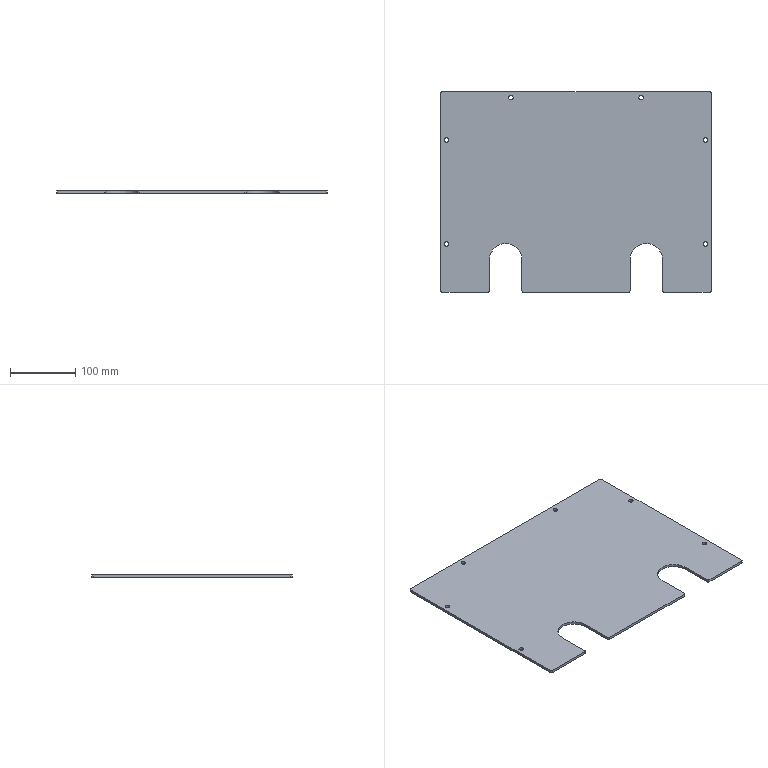Part | SolidWorks | features Fillet 2, HoleWzd 2, MirrorPattern 2, Extrusion 1, ICE 1 | 1 solid | 34 faces | box 416 x 308 x 4 mm | volume 483707 mm3 | cylinder 22 | plane 12 | commonest cylinder face diameters 7 x12 4 x8 50 x2
STEP:
#1=CARTESIAN_POINT('',(-103.5,145.,0.));
#2=VERTEX_POINT('',#1);
#3=CARTESIAN_POINT('',(-96.5,145.,0.));
#4=VERTEX_POINT('',#3);
#5=CARTESIAN_POINT('',(-100.,145.,0.));
#6=DIRECTION('',(0.,0.,1.));
#7=DIRECTION('',(1.,0.,0.));
#8=AXIS2_PLACEMENT_3D('',#5,#6,#7);
#9=CIRCLE('',#8,3.5);
#10=EDGE_CURVE('',#2,#4,#9,.T.);
#11=ORIENTED_EDGE('',*,*,#10,.F.);
#12=CARTESIAN_POINT('',(-103.5,145.,4.));
#13=VERTEX_POINT('',#12);
#14=CARTESIAN_POINT('',(-103.5,145.,4.));
#15=DIRECTION('',(0.,0.,1.));
#16=VECTOR('',#15,1000.);
#17=LINE('',#14,#16);
#18=EDGE_CURVE('',#2,#13,#17,.T.);
#19=ORIENTED_EDGE('',*,*,#18,.T.);
#20=CARTESIAN_POINT('',(-96.5,145.,4.));
#21=VERTEX_POINT('',#20);
#22=CARTESIAN_POINT('',(-100.,145.,4.));
#23=DIRECTION('',(0.,0.,1.));
#24=DIRECTION('',(1.,0.,0.));
#25=AXIS2_PLACEMENT_3D('',#22,#23,#24);
#26=CIRCLE('',#25,3.5);
#27=EDGE_CURVE('',#13,#21,#26,.T.);
#28=ORIENTED_EDGE('',*,*,#27,.T.);
#29=CARTESIAN_POINT('',(-96.5,145.,4.));
#30=DIRECTION('',(0.,0.,1.));
#31=VECTOR('',#30,1000.);
#32=LINE('',#29,#31);
#33=EDGE_CURVE('',#4,#21,#32,.T.);
#34=ORIENTED_EDGE('',*,*,#33,.F.);
#35=EDGE_LOOP('',(#11,#19,#28,#34));
#36=FACE_OUTER_BOUND('',#35,.T.);
#37=CARTESIAN_POINT('',(-100.,145.,4.));
#38=DIRECTION('',(0.,0.,1.));
#39=DIRECTION('',(1.,0.,0.));
#40=AXIS2_PLACEMENT_3D('',#37,#38,#39);
#41=CYLINDRICAL_SURFACE('',#40,3.5);
#42=ADVANCED_FACE('',(#36),#41,.F.);
#43=CARTESIAN_POINT('',(96.5,145.,0.));
#44=VERTEX_POINT('',#43);
#45=CARTESIAN_POINT('',(103.5,145.,0.));
#46=VERTEX_POINT('',#45);
#47=CARTESIAN_POINT('',(100.,145.,0.));
#48=DIRECTION('',(0.,0.,1.));
#49=DIRECTION('',(1.,0.,0.));
#50=AXIS2_PLACEMENT_3D('',#47,#48,#49);
#51=CIRCLE('',#50,3.5);
#52=EDGE_CURVE('',#44,#46,#51,.T.);
#53=ORIENTED_EDGE('',*,*,#52,.F.);
#54=CARTESIAN_POINT('',(96.5,145.,4.));
#55=VERTEX_POINT('',#54);
#56=CARTESIAN_POINT('',(96.5,145.,4.));
#57=DIRECTION('',(0.,0.,1.));
#58=VECTOR('',#57,1000.);
#59=LINE('',#56,#58);
#60=EDGE_CURVE('',#44,#55,#59,.T.);
#61=ORIENTED_EDGE('',*,*,#60,.T.);
#62=CARTESIAN_POINT('',(103.5,145.,4.));
#63=VERTEX_POINT('',#62);
#64=CARTESIAN_POINT('',(100.,145.,4.));
#65=DIRECTION('',(0.,0.,1.));
#66=DIRECTION('',(1.,0.,0.));
#67=AXIS2_PLACEMENT_3D('',#64,#65,#66);
#68=CIRCLE('',#67,3.5);
#69=EDGE_CURVE('',#55,#63,#68,.T.);
#70=ORIENTED_EDGE('',*,*,#69,.T.);
#71=CARTESIAN_POINT('',(103.5,145.,4.));
#72=DIRECTION('',(0.,0.,1.));
#73=VECTOR('',#72,1000.);
#74=LINE('',#71,#73);
#75=EDGE_CURVE('',#46,#63,#74,.T.);
#76=ORIENTED_EDGE('',*,*,#75,.F.);
#77=EDGE_LOOP('',(#53,#61,#70,#76));
#78=FACE_OUTER_BOUND('',#77,.T.);
#79=CARTESIAN_POINT('',(100.,145.,4.));
#80=DIRECTION('',(0.,0.,1.));
#81=DIRECTION('',(1.,0.,0.));
#82=AXIS2_PLACEMENT_3D('',#79,#80,#81);
#83=CYLINDRICAL_SURFACE('',#82,3.5);
#84=ADVANCED_FACE('',(#78),#83,.F.);
#85=CARTESIAN_POINT('',(195.5,80.,0.));
#86=VERTEX_POINT('',#85);
#87=CARTESIAN_POINT('',(202.5,80.,0.));
#88=VERTEX_POINT('',#87);
#89=CARTESIAN_POINT('',(199.,80.,0.));
#90=DIRECTION('',(0.,0.,1.));
#91=DIRECTION('',(1.,0.,0.));
#92=AXIS2_PLACEMENT_3D('',#89,#90,#91);
#93=CIRCLE('',#92,3.5);
#94=EDGE_CURVE('',#86,#88,#93,.T.);
#95=ORIENTED_EDGE('',*,*,#94,.F.);
#96=CARTESIAN_POINT('',(195.5,80.,4.));
#97=VERTEX_POINT('',#96);
#98=CARTESIAN_POINT('',(195.5,80.,4.));
#99=DIRECTION('',(0.,0.,1.));
#100=VECTOR('',#99,1000.);
#101=LINE('',#98,#100);
#102=EDGE_CURVE('',#86,#97,#101,.T.);
#103=ORIENTED_EDGE('',*,*,#102,.T.);
#104=CARTESIAN_POINT('',(202.5,80.,4.));
#105=VERTEX_POINT('',#104);
#106=CARTESIAN_POINT('',(199.,80.,4.));
#107=DIRECTION('',(0.,0.,1.));
#108=DIRECTION('',(1.,0.,0.));
#109=AXIS2_PLACEMENT_3D('',#106,#107,#108);
#110=CIRCLE('',#109,3.5);
#111=EDGE_CURVE('',#97,#105,#110,.T.);
#112=ORIENTED_EDGE('',*,*,#111,.T.);
#113=CARTESIAN_POINT('',(202.5,80.,4.));
#114=DIRECTION('',(0.,0.,1.));
#115=VECTOR('',#114,1000.);
#116=LINE('',#113,#115);
#117=EDGE_CURVE('',#88,#105,#116,.T.);
#118=ORIENTED_EDGE('',*,*,#117,.F.);
#119=EDGE_LOOP('',(#95,#103,#112,#118));
#120=FACE_OUTER_BOUND('',#119,.T.);
#121=CARTESIAN_POINT('',(199.,80.,4.));
#122=DIRECTION('',(0.,0.,1.));
#123=DIRECTION('',(1.,0.,0.));
#124=AXIS2_PLACEMENT_3D('',#121,#122,#123);
#125=CYLINDRICAL_SURFACE('',#124,3.5);
#126=ADVANCED_FACE('',(#120),#125,.F.);
#127=CARTESIAN_POINT('',(195.5,-80.,0.));
#128=VERTEX_POINT('',#127);
#129=CARTESIAN_POINT('',(202.5,-80.,0.));
#130=VERTEX_POINT('',#129);
#131=CARTESIAN_POINT('',(199.,-80.,0.));
#132=DIRECTION('',(0.,0.,1.));
#133=DIRECTION('',(1.,0.,0.));
#134=AXIS2_PLACEMENT_3D('',#131,#132,#133);
#135=CIRCLE('',#134,3.5);
#136=EDGE_CURVE('',#128,#130,#135,.T.);
#137=ORIENTED_EDGE('',*,*,#136,.F.);
#138=CARTESIAN_POINT('',(195.5,-80.,4.));
#139=VERTEX_POINT('',#138);
#140=CARTESIAN_POINT('',(195.5,-80.,4.));
#141=DIRECTION('',(0.,0.,1.));
#142=VECTOR('',#141,1000.);
#143=LINE('',#140,#142);
#144=EDGE_CURVE('',#128,#139,#143,.T.);
#145=ORIENTED_EDGE('',*,*,#144,.T.);
#146=CARTESIAN_POINT('',(202.5,-80.,4.));
#147=VERTEX_POINT('',#146);
#148=CARTESIAN_POINT('',(199.,-80.,4.));
#149=DIRECTION('',(0.,0.,1.));
#150=DIRECTION('',(1.,0.,0.));
#151=AXIS2_PLACEMENT_3D('',#148,#149,#150);
#152=CIRCLE('',#151,3.5);
#153=EDGE_CURVE('',#139,#147,#152,.T.);
#154=ORIENTED_EDGE('',*,*,#153,.T.);
#155=CARTESIAN_POINT('',(202.5,-80.,4.));
#156=DIRECTION('',(0.,0.,1.));
#157=VECTOR('',#156,1000.);
#158=LINE('',#155,#157);
#159=EDGE_CURVE('',#130,#147,#158,.T.);
#160=ORIENTED_EDGE('',*,*,#159,.F.);
#161=EDGE_LOOP('',(#137,#145,#154,#160));
#162=FACE_OUTER_BOUND('',#161,.T.);
#163=CARTESIAN_POINT('',(199.,-80.,4.));
#164=DIRECTION('',(0.,0.,1.));
#165=DIRECTION('',(1.,0.,0.));
#166=AXIS2_PLACEMENT_3D('',#163,#164,#165);
#167=CYLINDRICAL_SURFACE('',#166,3.5);
#168=ADVANCED_FACE('',(#162),#167,.F.);
#169=CARTESIAN_POINT('',(-202.5,80.,0.));
#170=VERTEX_POINT('',#169);
#171=CARTESIAN_POINT('',(-195.5,80.,0.));
#172=VERTEX_POINT('',#171);
#173=CARTESIAN_POINT('',(-199.,80.,0.));
#174=DIRECTION('',(0.,0.,1.));
#175=DIRECTION('',(1.,0.,0.));
#176=AXIS2_PLACEMENT_3D('',#173,#174,#175);
#177=CIRCLE('',#176,3.5);
#178=EDGE_CURVE('',#170,#172,#177,.T.);
#179=ORIENTED_EDGE('',*,*,#178,.F.);
#180=CARTESIAN_POINT('',(-202.5,80.,4.));
#181=VERTEX_POINT('',#180);
#182=CARTESIAN_POINT('',(-202.5,80.,4.));
#183=DIRECTION('',(0.,0.,1.));
#184=VECTOR('',#183,1000.);
#185=LINE('',#182,#184);
#186=EDGE_CURVE('',#170,#181,#185,.T.);
#187=ORIENTED_EDGE('',*,*,#186,.T.);
#188=CARTESIAN_POINT('',(-195.5,80.,4.));
#189=VERTEX_POINT('',#188);
#190=CARTESIAN_POINT('',(-199.,80.,4.));
#191=DIRECTION('',(0.,0.,1.));
#192=DIRECTION('',(1.,0.,0.));
#193=AXIS2_PLACEMENT_3D('',#190,#191,#192);
#194=CIRCLE('',#193,3.5);
#195=EDGE_CURVE('',#181,#189,#194,.T.);
#196=ORIENTED_EDGE('',*,*,#195,.T.);
#197=CARTESIAN_POINT('',(-195.5,80.,4.));
#198=DIRECTION('',(0.,0.,1.));
#199=VECTOR('',#198,1000.);
#200=LINE('',#197,#199);
#201=EDGE_CURVE('',#172,#189,#200,.T.);
#202=ORIENTED_EDGE('',*,*,#201,.F.);
#203=EDGE_LOOP('',(#179,#187,#196,#202));
#204=FACE_OUTER_BOUND('',#203,.T.);
#205=CARTESIAN_POINT('',(-199.,80.,4.));
#206=DIRECTION('',(0.,0.,1.));
#207=DIRECTION('',(1.,0.,0.));
#208=AXIS2_PLACEMENT_3D('',#205,#206,#207);
#209=CYLINDRICAL_SURFACE('',#208,3.5);
#210=ADVANCED_FACE('',(#204),#209,.F.);
#211=CARTESIAN_POINT('',(-202.5,-80.,0.));
#212=VERTEX_POINT('',#211);
#213=CARTESIAN_POINT('',(-195.5,-80.,0.));
#214=VERTEX_POINT('',#213);
#215=CARTESIAN_POINT('',(-199.,-80.,0.));
#216=DIRECTION('',(0.,0.,1.));
#217=DIRECTION('',(1.,0.,0.));
#218=AXIS2_PLACEMENT_3D('',#215,#216,#217);
#219=CIRCLE('',#218,3.5);
#220=EDGE_CURVE('',#212,#214,#219,.T.);
#221=ORIENTED_EDGE('',*,*,#220,.F.);
#222=CARTESIAN_POINT('',(-202.5,-80.,4.));
#223=VERTEX_POINT('',#222);
#224=CARTESIAN_POINT('',(-202.5,-80.,4.));
#225=DIRECTION('',(0.,0.,1.));
#226=VECTOR('',#225,1000.);
#227=LINE('',#224,#226);
#228=EDGE_CURVE('',#212,#223,#227,.T.);
#229=ORIENTED_EDGE('',*,*,#228,.T.);
#230=CARTESIAN_POINT('',(-195.5,-80.,4.));
#231=VERTEX_POINT('',#230);
#232=CARTESIAN_POINT('',(-199.,-80.,4.));
#233=DIRECTION('',(0.,0.,1.));
#234=DIRECTION('',(1.,0.,0.));
#235=AXIS2_PLACEMENT_3D('',#232,#233,#234);
#236=CIRCLE('',#235,3.5);
#237=EDGE_CURVE('',#223,#231,#236,.T.);
#238=ORIENTED_EDGE('',*,*,#237,.T.);
#239=CARTESIAN_POINT('',(-195.5,-80.,4.));
#240=DIRECTION('',(0.,0.,1.));
#241=VECTOR('',#240,1000.);
#242=LINE('',#239,#241);
#243=EDGE_CURVE('',#214,#231,#242,.T.);
#244=ORIENTED_EDGE('',*,*,#243,.F.);
#245=EDGE_LOOP('',(#221,#229,#238,#244));
#246=FACE_OUTER_BOUND('',#245,.T.);
#247=CARTESIAN_POINT('',(-199.,-80.,4.));
#248=DIRECTION('',(0.,0.,1.));
#249=DIRECTION('',(1.,0.,0.));
#250=AXIS2_PLACEMENT_3D('',#247,#248,#249);
#251=CYLINDRICAL_SURFACE('',#250,3.5);
#252=ADVANCED_FACE('',(#246),#251,.F.);
#253=CARTESIAN_POINT('',(-81.,-154.,0.));
#254=VERTEX_POINT('',#253);
#255=CARTESIAN_POINT('',(81.,-154.,0.));
#256=VERTEX_POINT('',#255);
#257=CARTESIAN_POINT('',(208.,-154.,0.));
#258=DIRECTION('',(1.,0.,0.));
#259=VECTOR('',#258,1000.);
#260=LINE('',#257,#259);
#261=EDGE_CURVE('',#254,#256,#260,.T.);
#262=ORIENTED_EDGE('',*,*,#261,.T.);
#263=CARTESIAN_POINT('',(81.,-154.,4.));
#264=VERTEX_POINT('',#263);
#265=CARTESIAN_POINT('',(81.,-154.,4.));
#266=DIRECTION('',(0.,0.,1.));
#267=VECTOR('',#266,1000.);
#268=LINE('',#265,#267);
#269=EDGE_CURVE('',#256,#264,#268,.T.);
#270=ORIENTED_EDGE('',*,*,#269,.T.);
#271=CARTESIAN_POINT('',(-81.,-154.,4.));
#272=VERTEX_POINT('',#271);
#273=CARTESIAN_POINT('',(208.,-154.,4.));
#274=DIRECTION('',(1.,0.,0.));
#275=VECTOR('',#274,1000.);
#276=LINE('',#273,#275);
#277=EDGE_CURVE('',#272,#264,#276,.T.);
#278=ORIENTED_EDGE('',*,*,#277,.F.);
#279=CARTESIAN_POINT('',(-81.,-154.,4.));
#280=DIRECTION('',(0.,0.,-1.));
#281=VECTOR('',#280,1000.);
#282=LINE('',#279,#281);
#283=EDGE_CURVE('',#272,#254,#282,.T.);
#284=ORIENTED_EDGE('',*,*,#283,.T.);
#285=EDGE_LOOP('',(#262,#270,#278,#284));
#286=FACE_OUTER_BOUND('',#285,.T.);
#287=CARTESIAN_POINT('',(208.,-154.,4.));
#288=DIRECTION('',(0.,1.,0.));
#289=DIRECTION('',(-1.,0.,0.));
#290=AXIS2_PLACEMENT_3D('',#287,#288,#289);
#291=PLANE('',#290);
#292=ADVANCED_FACE('',(#286),#291,.F.);
#293=CARTESIAN_POINT('',(135.,-154.,4.));
#294=VERTEX_POINT('',#293);
#295=CARTESIAN_POINT('',(206.,-154.,4.));
#296=VERTEX_POINT('',#295);
#297=CARTESIAN_POINT('',(208.,-154.,4.));
#298=DIRECTION('',(1.,0.,0.));
#299=VECTOR('',#298,1000.);
#300=LINE('',#297,#299);
#301=EDGE_CURVE('',#294,#296,#300,.T.);
#302=ORIENTED_EDGE('',*,*,#301,.F.);
#303=CARTESIAN_POINT('',(135.,-154.,0.));
#304=VERTEX_POINT('',#303);
#305=CARTESIAN_POINT('',(135.,-154.,0.));
#306=DIRECTION('',(0.,0.,-1.));
#307=VECTOR('',#306,1000.);
#308=LINE('',#305,#307);
#309=EDGE_CURVE('',#294,#304,#308,.T.);
#310=ORIENTED_EDGE('',*,*,#309,.T.);
#311=CARTESIAN_POINT('',(206.,-154.,0.));
#312=VERTEX_POINT('',#311);
#313=CARTESIAN_POINT('',(208.,-154.,0.));
#314=DIRECTION('',(1.,0.,0.));
#315=VECTOR('',#314,1000.);
#316=LINE('',#313,#315);
#317=EDGE_CURVE('',#304,#312,#316,.T.);
#318=ORIENTED_EDGE('',*,*,#317,.T.);
#319=CARTESIAN_POINT('',(206.,-154.,4.));
#320=DIRECTION('',(0.,0.,1.));
#321=VECTOR('',#320,1000.);
#322=LINE('',#319,#321);
#323=EDGE_CURVE('',#312,#296,#322,.T.);
#324=ORIENTED_EDGE('',*,*,#323,.T.);
#325=EDGE_LOOP('',(#302,#310,#318,#324));
#326=FACE_OUTER_BOUND('',#325,.T.);
#327=CARTESIAN_POINT('',(208.,-154.,4.));
#328=DIRECTION('',(0.,1.,0.));
#329=DIRECTION('',(-1.,0.,0.));
#330=AXIS2_PLACEMENT_3D('',#327,#328,#329);
#331=PLANE('',#330);
#332=ADVANCED_FACE('',(#326),#331,.F.);
#333=CARTESIAN_POINT('',(-100.,145.,4.));
#334=DIRECTION('',(0.,0.,1.));
#335=DIRECTION('',(1.,0.,0.));
#336=AXIS2_PLACEMENT_3D('',#333,#334,#335);
#337=CIRCLE('',#336,3.5);
#338=EDGE_CURVE('',#21,#13,#337,.T.);
#339=ORIENTED_EDGE('',*,*,#338,.F.);
#340=ORIENTED_EDGE('',*,*,#27,.F.);
#341=EDGE_LOOP('',(#339,#340));
#342=FACE_BOUND('',#341,.T.);
#343=CARTESIAN_POINT('',(100.,145.,4.));
#344=DIRECTION('',(0.,0.,1.));
#345=DIRECTION('',(1.,0.,0.));
#346=AXIS2_PLACEMENT_3D('',#343,#344,#345);
#347=CIRCLE('',#346,3.5);
#348=EDGE_CURVE('',#63,#55,#347,.T.);
#349=ORIENTED_EDGE('',*,*,#348,.F.);
#350=ORIENTED_EDGE('',*,*,#69,.F.);
#351=EDGE_LOOP('',(#349,#350));
#352=FACE_BOUND('',#351,.T.);
#353=CARTESIAN_POINT('',(199.,80.,4.));
#354=DIRECTION('',(0.,0.,1.));
#355=DIRECTION('',(1.,0.,0.));
#356=AXIS2_PLACEMENT_3D('',#353,#354,#355);
#357=CIRCLE('',#356,3.5);
#358=EDGE_CURVE('',#105,#97,#357,.T.);
#359=ORIENTED_EDGE('',*,*,#358,.F.);
#360=ORIENTED_EDGE('',*,*,#111,.F.);
#361=EDGE_LOOP('',(#359,#360));
#362=FACE_BOUND('',#361,.T.);
#363=CARTESIAN_POINT('',(199.,-80.,4.));
#364=DIRECTION('',(0.,0.,1.));
#365=DIRECTION('',(1.,0.,0.));
#366=AXIS2_PLACEMENT_3D('',#363,#364,#365);
#367=CIRCLE('',#366,3.5);
#368=EDGE_CURVE('',#147,#139,#367,.T.);
#369=ORIENTED_EDGE('',*,*,#368,.F.);
#370=ORIENTED_EDGE('',*,*,#153,.F.);
#371=EDGE_LOOP('',(#369,#370));
#372=FACE_BOUND('',#371,.T.);
#373=CARTESIAN_POINT('',(-199.,80.,4.));
#374=DIRECTION('',(0.,0.,1.));
#375=DIRECTION('',(1.,0.,0.));
#376=AXIS2_PLACEMENT_3D('',#373,#374,#375);
#377=CIRCLE('',#376,3.5);
#378=EDGE_CURVE('',#189,#181,#377,.T.);
#379=ORIENTED_EDGE('',*,*,#378,.F.);
#380=ORIENTED_EDGE('',*,*,#195,.F.);
#381=EDGE_LOOP('',(#379,#380));
#382=FACE_BOUND('',#381,.T.);
#383=CARTESIAN_POINT('',(-199.,-80.,4.));
#384=DIRECTION('',(0.,0.,1.));
#385=DIRECTION('',(1.,0.,0.));
#386=AXIS2_PLACEMENT_3D('',#383,#384,#385);
#387=CIRCLE('',#386,3.5);
#388=EDGE_CURVE('',#231,#223,#387,.T.);
#389=ORIENTED_EDGE('',*,*,#388,.F.);
#390=ORIENTED_EDGE('',*,*,#237,.F.);
#391=EDGE_LOOP('',(#389,#390));
#392=FACE_BOUND('',#391,.T.);
#393=CARTESIAN_POINT('',(133.,-104.,4.));
#394=VERTEX_POINT('',#393);
#395=CARTESIAN_POINT('',(133.,-152.,4.));
#396=VERTEX_POINT('',#395);
#397=CARTESIAN_POINT('',(133.,-154.,4.));
#398=DIRECTION('',(0.,-1.,0.));
#399=VECTOR('',#398,1000.);
#400=LINE('',#397,#399);
#401=EDGE_CURVE('',#394,#396,#400,.T.);
#402=ORIENTED_EDGE('',*,*,#401,.T.);
#403=CARTESIAN_POINT('',(135.,-152.,4.));
#404=DIRECTION('',(0.,0.,1.));
#405=DIRECTION('',(1.,0.,0.));
#406=AXIS2_PLACEMENT_3D('',#403,#404,#405);
#407=CIRCLE('',#406,2.);
#408=EDGE_CURVE('',#396,#294,#407,.T.);
#409=ORIENTED_EDGE('',*,*,#408,.T.);
#410=ORIENTED_EDGE('',*,*,#301,.T.);
#411=CARTESIAN_POINT('',(208.,-152.,4.));
#412=VERTEX_POINT('',#411);
#413=CARTESIAN_POINT('',(206.,-152.,4.));
#414=DIRECTION('',(0.,0.,1.));
#415=DIRECTION('',(1.,0.,0.));
#416=AXIS2_PLACEMENT_3D('',#413,#414,#415);
#417=CIRCLE('',#416,2.);
#418=EDGE_CURVE('',#296,#412,#417,.T.);
#419=ORIENTED_EDGE('',*,*,#418,.T.);
#420=CARTESIAN_POINT('',(208.,152.,4.));
#421=VERTEX_POINT('',#420);
#422=CARTESIAN_POINT('',(208.,-154.,4.));
#423=DIRECTION('',(0.,1.,0.));
#424=VECTOR('',#423,1000.);
#425=LINE('',#422,#424);
#426=EDGE_CURVE('',#412,#421,#425,.T.);
#427=ORIENTED_EDGE('',*,*,#426,.T.);
#428=CARTESIAN_POINT('',(206.,154.,4.));
#429=VERTEX_POINT('',#428);
#430=CARTESIAN_POINT('',(206.,152.,4.));
#431=DIRECTION('',(0.,0.,1.));
#432=DIRECTION('',(1.,0.,0.));
#433=AXIS2_PLACEMENT_3D('',#430,#431,#432);
#434=CIRCLE('',#433,2.);
#435=EDGE_CURVE('',#421,#429,#434,.T.);
#436=ORIENTED_EDGE('',*,*,#435,.T.);
#437=CARTESIAN_POINT('',(-206.,154.,4.));
#438=VERTEX_POINT('',#437);
#439=CARTESIAN_POINT('',(208.,154.,4.));
#440=DIRECTION('',(-1.,0.,0.));
#441=VECTOR('',#440,1000.);
#442=LINE('',#439,#441);
#443=EDGE_CURVE('',#429,#438,#442,.T.);
#444=ORIENTED_EDGE('',*,*,#443,.T.);
#445=CARTESIAN_POINT('',(-208.,152.,4.));
#446=VERTEX_POINT('',#445);
#447=CARTESIAN_POINT('',(-206.,152.,4.));
#448=DIRECTION('',(0.,0.,1.));
#449=DIRECTION('',(1.,0.,0.));
#450=AXIS2_PLACEMENT_3D('',#447,#448,#449);
#451=CIRCLE('',#450,2.);
#452=EDGE_CURVE('',#438,#446,#451,.T.);
#453=ORIENTED_EDGE('',*,*,#452,.T.);
#454=CARTESIAN_POINT('',(-208.,-152.,4.));
#455=VERTEX_POINT('',#454);
#456=CARTESIAN_POINT('',(-208.,-154.,4.));
#457=DIRECTION('',(0.,-1.,0.));
#458=VECTOR('',#457,1000.);
#459=LINE('',#456,#458);
#460=EDGE_CURVE('',#446,#455,#459,.T.);
#461=ORIENTED_EDGE('',*,*,#460,.T.);
#462=CARTESIAN_POINT('',(-206.,-154.,4.));
#463=VERTEX_POINT('',#462);
#464=CARTESIAN_POINT('',(-206.,-152.,4.));
#465=DIRECTION('',(0.,0.,1.));
#466=DIRECTION('',(1.,0.,0.));
#467=AXIS2_PLACEMENT_3D('',#464,#465,#466);
#468=CIRCLE('',#467,2.);
#469=EDGE_CURVE('',#455,#463,#468,.T.);
#470=ORIENTED_EDGE('',*,*,#469,.T.);
#471=CARTESIAN_POINT('',(-135.,-154.,4.));
#472=VERTEX_POINT('',#471);
#473=CARTESIAN_POINT('',(208.,-154.,4.));
#474=DIRECTION('',(1.,0.,0.));
#475=VECTOR('',#474,1000.);
#476=LINE('',#473,#475);
#477=EDGE_CURVE('',#463,#472,#476,.T.);
#478=ORIENTED_EDGE('',*,*,#477,.T.);
#479=CARTESIAN_POINT('',(-133.,-152.,4.));
#480=VERTEX_POINT('',#479);
#481=CARTESIAN_POINT('',(-135.,-152.,4.));
#482=DIRECTION('',(0.,0.,1.));
#483=DIRECTION('',(1.,0.,0.));
#484=AXIS2_PLACEMENT_3D('',#481,#482,#483);
#485=CIRCLE('',#484,2.);
#486=EDGE_CURVE('',#472,#480,#485,.T.);
#487=ORIENTED_EDGE('',*,*,#486,.T.);
#488=CARTESIAN_POINT('',(-133.,-104.,4.));
#489=VERTEX_POINT('',#488);
#490=CARTESIAN_POINT('',(-133.,-154.,4.));
#491=DIRECTION('',(0.,-1.,0.));
#492=VECTOR('',#491,1000.);
#493=LINE('',#490,#492);
#494=EDGE_CURVE('',#489,#480,#493,.T.);
#495=ORIENTED_EDGE('',*,*,#494,.F.);
#496=CARTESIAN_POINT('',(-83.,-104.,4.));
#497=VERTEX_POINT('',#496);
#498=CARTESIAN_POINT('',(-108.,-104.,4.));
#499=DIRECTION('',(0.,0.,1.));
#500=DIRECTION('',(1.,0.,0.));
#501=AXIS2_PLACEMENT_3D('',#498,#499,#500);
#502=CIRCLE('',#501,25.);
#503=EDGE_CURVE('',#497,#489,#502,.T.);
#504=ORIENTED_EDGE('',*,*,#503,.F.);
#505=CARTESIAN_POINT('',(-83.,-152.,4.));
#506=VERTEX_POINT('',#505);
#507=CARTESIAN_POINT('',(-83.,-154.,4.));
#508=DIRECTION('',(0.,1.,0.));
#509=VECTOR('',#508,1000.);
#510=LINE('',#507,#509);
#511=EDGE_CURVE('',#506,#497,#510,.T.);
#512=ORIENTED_EDGE('',*,*,#511,.F.);
#513=CARTESIAN_POINT('',(-81.,-152.,4.));
#514=DIRECTION('',(0.,0.,1.));
#515=DIRECTION('',(1.,0.,0.));
#516=AXIS2_PLACEMENT_3D('',#513,#514,#515);
#517=CIRCLE('',#516,2.);
#518=EDGE_CURVE('',#506,#272,#517,.T.);
#519=ORIENTED_EDGE('',*,*,#518,.T.);
#520=ORIENTED_EDGE('',*,*,#277,.T.);
#521=CARTESIAN_POINT('',(83.,-152.,4.));
#522=VERTEX_POINT('',#521);
#523=CARTESIAN_POINT('',(81.,-152.,4.));
#524=DIRECTION('',(0.,0.,1.));
#525=DIRECTION('',(1.,0.,0.));
#526=AXIS2_PLACEMENT_3D('',#523,#524,#525);
#527=CIRCLE('',#526,2.);
#528=EDGE_CURVE('',#264,#522,#527,.T.);
#529=ORIENTED_EDGE('',*,*,#528,.T.);
#530=CARTESIAN_POINT('',(83.,-104.,4.));
#531=VERTEX_POINT('',#530);
#532=CARTESIAN_POINT('',(83.,-154.,4.));
#533=DIRECTION('',(0.,1.,0.));
#534=VECTOR('',#533,1000.);
#535=LINE('',#532,#534);
#536=EDGE_CURVE('',#522,#531,#535,.T.);
#537=ORIENTED_EDGE('',*,*,#536,.T.);
#538=CARTESIAN_POINT('',(108.,-104.,4.));
#539=DIRECTION('',(0.,0.,-1.));
#540=DIRECTION('',(-1.,0.,0.));
#541=AXIS2_PLACEMENT_3D('',#538,#539,#540);
#542=CIRCLE('',#541,25.);
#543=EDGE_CURVE('',#531,#394,#542,.T.);
#544=ORIENTED_EDGE('',*,*,#543,.T.);
#545=EDGE_LOOP('',(#402,#409,#410,#419,#427,#436,#444,#453,#461,#470,#478,#487,#495,#504,#512,#519,#520,#529,#537,#544));
#546=FACE_OUTER_BOUND('',#545,.T.);
#547=CARTESIAN_POINT('',(0.,0.,4.));
#548=DIRECTION('',(0.,0.,1.));
#549=DIRECTION('',(1.,0.,0.));
#550=AXIS2_PLACEMENT_3D('',#547,#548,#549);
#551=PLANE('',#550);
#552=ADVANCED_FACE('',(#342,#352,#362,#372,#382,#392,#546),#551,.T.);
#553=CARTESIAN_POINT('',(-100.,145.,0.));
#554=DIRECTION('',(0.,0.,1.));
#555=DIRECTION('',(1.,0.,0.));
#556=AXIS2_PLACEMENT_3D('',#553,#554,#555);
#557=CIRCLE('',#556,3.5);
#558=EDGE_CURVE('',#4,#2,#557,.T.);
#559=ORIENTED_EDGE('',*,*,#558,.T.);
#560=ORIENTED_EDGE('',*,*,#10,.T.);
#561=EDGE_LOOP('',(#559,#560));
#562=FACE_BOUND('',#561,.T.);
#563=CARTESIAN_POINT('',(100.,145.,0.));
#564=DIRECTION('',(0.,0.,1.));
#565=DIRECTION('',(1.,0.,0.));
#566=AXIS2_PLACEMENT_3D('',#563,#564,#565);
#567=CIRCLE('',#566,3.5);
#568=EDGE_CURVE('',#46,#44,#567,.T.);
#569=ORIENTED_EDGE('',*,*,#568,.T.);
#570=ORIENTED_EDGE('',*,*,#52,.T.);
#571=EDGE_LOOP('',(#569,#570));
#572=FACE_BOUND('',#571,.T.);
#573=CARTESIAN_POINT('',(199.,80.,0.));
#574=DIRECTION('',(0.,0.,1.));
#575=DIRECTION('',(1.,0.,0.));
#576=AXIS2_PLACEMENT_3D('',#573,#574,#575);
#577=CIRCLE('',#576,3.5);
#578=EDGE_CURVE('',#88,#86,#577,.T.);
#579=ORIENTED_EDGE('',*,*,#578,.T.);
#580=ORIENTED_EDGE('',*,*,#94,.T.);
#581=EDGE_LOOP('',(#579,#580));
#582=FACE_BOUND('',#581,.T.);
#583=CARTESIAN_POINT('',(199.,-80.,0.));
#584=DIRECTION('',(0.,0.,1.));
#585=DIRECTION('',(1.,0.,0.));
#586=AXIS2_PLACEMENT_3D('',#583,#584,#585);
#587=CIRCLE('',#586,3.5);
#588=EDGE_CURVE('',#130,#128,#587,.T.);
#589=ORIENTED_EDGE('',*,*,#588,.T.);
#590=ORIENTED_EDGE('',*,*,#136,.T.);
#591=EDGE_LOOP('',(#589,#590));
#592=FACE_BOUND('',#591,.T.);
#593=CARTESIAN_POINT('',(-199.,80.,0.));
#594=DIRECTION('',(0.,0.,1.));
#595=DIRECTION('',(1.,0.,0.));
#596=AXIS2_PLACEMENT_3D('',#593,#594,#595);
#597=CIRCLE('',#596,3.5);
#598=EDGE_CURVE('',#172,#170,#597,.T.);
#599=ORIENTED_EDGE('',*,*,#598,.T.);
#600=ORIENTED_EDGE('',*,*,#178,.T.);
#601=EDGE_LOOP('',(#599,#600));
#602=FACE_BOUND('',#601,.T.);
#603=CARTESIAN_POINT('',(-199.,-80.,0.));
#604=DIRECTION('',(0.,0.,1.));
#605=DIRECTION('',(1.,0.,0.));
#606=AXIS2_PLACEMENT_3D('',#603,#604,#605);
#607=CIRCLE('',#606,3.5);
#608=EDGE_CURVE('',#214,#212,#607,.T.);
#609=ORIENTED_EDGE('',*,*,#608,.T.);
#610=ORIENTED_EDGE('',*,*,#220,.T.);
#611=EDGE_LOOP('',(#609,#610));
#612=FACE_BOUND('',#611,.T.);
#613=ORIENTED_EDGE('',*,*,#317,.F.);
#614=CARTESIAN_POINT('',(133.,-152.,0.));
#615=VERTEX_POINT('',#614);
#616=CARTESIAN_POINT('',(135.,-152.,0.));
#617=DIRECTION('',(0.,0.,-1.));
#618=DIRECTION('',(1.,0.,0.));
#619=AXIS2_PLACEMENT_3D('',#616,#617,#618);
#620=CIRCLE('',#619,2.);
#621=EDGE_CURVE('',#304,#615,#620,.T.);
#622=ORIENTED_EDGE('',*,*,#621,.T.);
#623=CARTESIAN_POINT('',(133.,-104.,0.));
#624=VERTEX_POINT('',#623);
#625=CARTESIAN_POINT('',(133.,-154.,0.));
#626=DIRECTION('',(0.,1.,0.));
#627=VECTOR('',#626,1000.);
#628=LINE('',#625,#627);
#629=EDGE_CURVE('',#615,#624,#628,.T.);
#630=ORIENTED_EDGE('',*,*,#629,.T.);
#631=CARTESIAN_POINT('',(83.,-104.,0.));
#632=VERTEX_POINT('',#631);
#633=CARTESIAN_POINT('',(108.,-104.,0.));
#634=DIRECTION('',(0.,0.,1.));
#635=DIRECTION('',(1.,0.,0.));
#636=AXIS2_PLACEMENT_3D('',#633,#634,#635);
#637=CIRCLE('',#636,25.);
#638=EDGE_CURVE('',#624,#632,#637,.T.);
#639=ORIENTED_EDGE('',*,*,#638,.T.);
#640=CARTESIAN_POINT('',(83.,-152.,0.));
#641=VERTEX_POINT('',#640);
#642=CARTESIAN_POINT('',(83.,-154.,0.));
#643=DIRECTION('',(0.,-1.,0.));
#644=VECTOR('',#643,1000.);
#645=LINE('',#642,#644);
#646=EDGE_CURVE('',#632,#641,#645,.T.);
#647=ORIENTED_EDGE('',*,*,#646,.T.);
#648=CARTESIAN_POINT('',(81.,-152.,0.));
#649=DIRECTION('',(0.,0.,-1.));
#650=DIRECTION('',(1.,0.,0.));
#651=AXIS2_PLACEMENT_3D('',#648,#649,#650);
#652=CIRCLE('',#651,2.);
#653=EDGE_CURVE('',#641,#256,#652,.T.);
#654=ORIENTED_EDGE('',*,*,#653,.T.);
#655=ORIENTED_EDGE('',*,*,#261,.F.);
#656=CARTESIAN_POINT('',(-83.,-152.,0.));
#657=VERTEX_POINT('',#656);
#658=CARTESIAN_POINT('',(-81.,-152.,0.));
#659=DIRECTION('',(0.,0.,-1.));
#660=DIRECTION('',(1.,0.,0.));
#661=AXIS2_PLACEMENT_3D('',#658,#659,#660);
#662=CIRCLE('',#661,2.);
#663=EDGE_CURVE('',#254,#657,#662,.T.);
#664=ORIENTED_EDGE('',*,*,#663,.T.);
#665=CARTESIAN_POINT('',(-83.,-104.,0.));
#666=VERTEX_POINT('',#665);
#667=CARTESIAN_POINT('',(-83.,-154.,0.));
#668=DIRECTION('',(0.,-1.,0.));
#669=VECTOR('',#668,1000.);
#670=LINE('',#667,#669);
#671=EDGE_CURVE('',#666,#657,#670,.T.);
#672=ORIENTED_EDGE('',*,*,#671,.F.);
#673=CARTESIAN_POINT('',(-133.,-104.,0.));
#674=VERTEX_POINT('',#673);
#675=CARTESIAN_POINT('',(-108.,-104.,0.));
#676=DIRECTION('',(0.,0.,-1.));
#677=DIRECTION('',(1.,0.,0.));
#678=AXIS2_PLACEMENT_3D('',#675,#676,#677);
#679=CIRCLE('',#678,25.);
#680=EDGE_CURVE('',#674,#666,#679,.T.);
#681=ORIENTED_EDGE('',*,*,#680,.F.);
#682=CARTESIAN_POINT('',(-133.,-152.,0.));
#683=VERTEX_POINT('',#682);
#684=CARTESIAN_POINT('',(-133.,-154.,0.));
#685=DIRECTION('',(0.,1.,0.));
#686=VECTOR('',#685,1000.);
#687=LINE('',#684,#686);
#688=EDGE_CURVE('',#683,#674,#687,.T.);
#689=ORIENTED_EDGE('',*,*,#688,.F.);
#690=CARTESIAN_POINT('',(-135.,-154.,0.));
#691=VERTEX_POINT('',#690);
#692=CARTESIAN_POINT('',(-135.,-152.,0.));
#693=DIRECTION('',(0.,0.,-1.));
#694=DIRECTION('',(1.,0.,0.));
#695=AXIS2_PLACEMENT_3D('',#692,#693,#694);
#696=CIRCLE('',#695,2.);
#697=EDGE_CURVE('',#683,#691,#696,.T.);
#698=ORIENTED_EDGE('',*,*,#697,.T.);
#699=CARTESIAN_POINT('',(-206.,-154.,0.));
#700=VERTEX_POINT('',#699);
#701=CARTESIAN_POINT('',(208.,-154.,0.));
#702=DIRECTION('',(1.,0.,0.));
#703=VECTOR('',#702,1000.);
#704=LINE('',#701,#703);
#705=EDGE_CURVE('',#700,#691,#704,.T.);
#706=ORIENTED_EDGE('',*,*,#705,.F.);
#707=CARTESIAN_POINT('',(-208.,-152.,0.));
#708=VERTEX_POINT('',#707);
#709=CARTESIAN_POINT('',(-206.,-152.,0.));
#710=DIRECTION('',(0.,0.,-1.));
#711=DIRECTION('',(1.,0.,0.));
#712=AXIS2_PLACEMENT_3D('',#709,#710,#711);
#713=CIRCLE('',#712,2.);
#714=EDGE_CURVE('',#700,#708,#713,.T.);
#715=ORIENTED_EDGE('',*,*,#714,.T.);
#716=CARTESIAN_POINT('',(-208.,152.,0.));
#717=VERTEX_POINT('',#716);
#718=CARTESIAN_POINT('',(-208.,-154.,0.));
#719=DIRECTION('',(0.,-1.,0.));
#720=VECTOR('',#719,1000.);
#721=LINE('',#718,#720);
#722=EDGE_CURVE('',#717,#708,#721,.T.);
#723=ORIENTED_EDGE('',*,*,#722,.F.);
#724=CARTESIAN_POINT('',(-206.,154.,0.));
#725=VERTEX_POINT('',#724);
#726=CARTESIAN_POINT('',(-206.,152.,0.));
#727=DIRECTION('',(0.,0.,-1.));
#728=DIRECTION('',(1.,0.,0.));
#729=AXIS2_PLACEMENT_3D('',#726,#727,#728);
#730=CIRCLE('',#729,2.);
#731=EDGE_CURVE('',#717,#725,#730,.T.);
#732=ORIENTED_EDGE('',*,*,#731,.T.);
#733=CARTESIAN_POINT('',(206.,154.,0.));
#734=VERTEX_POINT('',#733);
#735=CARTESIAN_POINT('',(208.,154.,0.));
#736=DIRECTION('',(-1.,0.,0.));
#737=VECTOR('',#736,1000.);
#738=LINE('',#735,#737);
#739=EDGE_CURVE('',#734,#725,#738,.T.);
#740=ORIENTED_EDGE('',*,*,#739,.F.);
#741=CARTESIAN_POINT('',(208.,152.,0.));
#742=VERTEX_POINT('',#741);
#743=CARTESIAN_POINT('',(206.,152.,0.));
#744=DIRECTION('',(0.,0.,-1.));
#745=DIRECTION('',(1.,0.,0.));
#746=AXIS2_PLACEMENT_3D('',#743,#744,#745);
#747=CIRCLE('',#746,2.);
#748=EDGE_CURVE('',#734,#742,#747,.T.);
#749=ORIENTED_EDGE('',*,*,#748,.T.);
#750=CARTESIAN_POINT('',(208.,-152.,0.));
#751=VERTEX_POINT('',#750);
#752=CARTESIAN_POINT('',(208.,-154.,0.));
#753=DIRECTION('',(0.,1.,0.));
#754=VECTOR('',#753,1000.);
#755=LINE('',#752,#754);
#756=EDGE_CURVE('',#751,#742,#755,.T.);
#757=ORIENTED_EDGE('',*,*,#756,.F.);
#758=CARTESIAN_POINT('',(206.,-152.,0.));
#759=DIRECTION('',(0.,0.,-1.));
#760=DIRECTION('',(1.,0.,0.));
#761=AXIS2_PLACEMENT_3D('',#758,#759,#760);
#762=CIRCLE('',#761,2.);
#763=EDGE_CURVE('',#751,#312,#762,.T.);
#764=ORIENTED_EDGE('',*,*,#763,.T.);
#765=EDGE_LOOP('',(#613,#622,#630,#639,#647,#654,#655,#664,#672,#681,#689,#698,#706,#715,#723,#732,#740,#749,#757,#764));
#766=FACE_OUTER_BOUND('',#765,.T.);
#767=CARTESIAN_POINT('',(0.,0.,0.));
#768=DIRECTION('',(0.,0.,1.));
#769=DIRECTION('',(1.,0.,0.));
#770=AXIS2_PLACEMENT_3D('',#767,#768,#769);
#771=PLANE('',#770);
#772=ADVANCED_FACE('',(#562,#572,#582,#592,#602,#612,#766),#771,.F.);
#773=ORIENTED_EDGE('',*,*,#705,.T.);
#774=CARTESIAN_POINT('',(-135.,-154.,4.));
#775=DIRECTION('',(0.,0.,1.));
#776=VECTOR('',#775,1000.);
#777=LINE('',#774,#776);
#778=EDGE_CURVE('',#691,#472,#777,.T.);
#779=ORIENTED_EDGE('',*,*,#778,.T.);
#780=ORIENTED_EDGE('',*,*,#477,.F.);
#781=CARTESIAN_POINT('',(-206.,-154.,4.));
#782=DIRECTION('',(0.,0.,-1.));
#783=VECTOR('',#782,1000.);
#784=LINE('',#781,#783);
#785=EDGE_CURVE('',#463,#700,#784,.T.);
#786=ORIENTED_EDGE('',*,*,#785,.T.);
#787=EDGE_LOOP('',(#773,#779,#780,#786));
#788=FACE_OUTER_BOUND('',#787,.T.);
#789=CARTESIAN_POINT('',(208.,-154.,4.));
#790=DIRECTION('',(0.,1.,0.));
#791=DIRECTION('',(-1.,0.,0.));
#792=AXIS2_PLACEMENT_3D('',#789,#790,#791);
#793=PLANE('',#792);
#794=ADVANCED_FACE('',(#788),#793,.F.);
#795=ORIENTED_EDGE('',*,*,#722,.T.);
#796=CARTESIAN_POINT('',(-208.,-152.,4.));
#797=DIRECTION('',(0.,0.,1.));
#798=VECTOR('',#797,1000.);
#799=LINE('',#796,#798);
#800=EDGE_CURVE('',#708,#455,#799,.T.);
#801=ORIENTED_EDGE('',*,*,#800,.T.);
#802=ORIENTED_EDGE('',*,*,#460,.F.);
#803=CARTESIAN_POINT('',(-208.,152.,4.));
#804=DIRECTION('',(0.,0.,-1.));
#805=VECTOR('',#804,1000.);
#806=LINE('',#803,#805);
#807=EDGE_CURVE('',#446,#717,#806,.T.);
#808=ORIENTED_EDGE('',*,*,#807,.T.);
#809=EDGE_LOOP('',(#795,#801,#802,#808));
#810=FACE_OUTER_BOUND('',#809,.T.);
#811=CARTESIAN_POINT('',(-208.,-154.,4.));
#812=DIRECTION('',(1.,0.,0.));
#813=DIRECTION('',(0.,0.,-1.));
#814=AXIS2_PLACEMENT_3D('',#811,#812,#813);
#815=PLANE('',#814);
#816=ADVANCED_FACE('',(#810),#815,.F.);
#817=ORIENTED_EDGE('',*,*,#756,.T.);
#818=CARTESIAN_POINT('',(208.,152.,4.));
#819=DIRECTION('',(0.,0.,1.));
#820=VECTOR('',#819,1000.);
#821=LINE('',#818,#820);
#822=EDGE_CURVE('',#742,#421,#821,.T.);
#823=ORIENTED_EDGE('',*,*,#822,.T.);
#824=ORIENTED_EDGE('',*,*,#426,.F.);
#825=CARTESIAN_POINT('',(208.,-152.,4.));
#826=DIRECTION('',(0.,0.,-1.));
#827=VECTOR('',#826,1000.);
#828=LINE('',#825,#827);
#829=EDGE_CURVE('',#412,#751,#828,.T.);
#830=ORIENTED_EDGE('',*,*,#829,.T.);
#831=EDGE_LOOP('',(#817,#823,#824,#830));
#832=FACE_OUTER_BOUND('',#831,.T.);
#833=CARTESIAN_POINT('',(208.,-154.,4.));
#834=DIRECTION('',(-1.,0.,0.));
#835=DIRECTION('',(0.,0.,1.));
#836=AXIS2_PLACEMENT_3D('',#833,#834,#835);
#837=PLANE('',#836);
#838=ADVANCED_FACE('',(#832),#837,.F.);
#839=ORIENTED_EDGE('',*,*,#443,.F.);
#840=CARTESIAN_POINT('',(206.,154.,4.));
#841=DIRECTION('',(0.,0.,-1.));
#842=VECTOR('',#841,1000.);
#843=LINE('',#840,#842);
#844=EDGE_CURVE('',#429,#734,#843,.T.);
#845=ORIENTED_EDGE('',*,*,#844,.T.);
#846=ORIENTED_EDGE('',*,*,#739,.T.);
#847=CARTESIAN_POINT('',(-206.,154.,4.));
#848=DIRECTION('',(0.,0.,1.));
#849=VECTOR('',#848,1000.);
#850=LINE('',#847,#849);
#851=EDGE_CURVE('',#725,#438,#850,.T.);
#852=ORIENTED_EDGE('',*,*,#851,.T.);
#853=EDGE_LOOP('',(#839,#845,#846,#852));
#854=FACE_OUTER_BOUND('',#853,.T.);
#855=CARTESIAN_POINT('',(208.,154.,4.));
#856=DIRECTION('',(0.,-1.,0.));
#857=DIRECTION('',(1.,0.,0.));
#858=AXIS2_PLACEMENT_3D('',#855,#856,#857);
#859=PLANE('',#858);
#860=ADVANCED_FACE('',(#854),#859,.F.);
#861=ORIENTED_EDGE('',*,*,#435,.F.);
#862=ORIENTED_EDGE('',*,*,#822,.F.);
#863=ORIENTED_EDGE('',*,*,#748,.F.);
#864=ORIENTED_EDGE('',*,*,#844,.F.);
#865=EDGE_LOOP('',(#861,#862,#863,#864));
#866=FACE_OUTER_BOUND('',#865,.T.);
#867=CARTESIAN_POINT('',(206.,152.,4.));
#868=DIRECTION('',(0.,0.,-1.));
#869=DIRECTION('',(-1.,0.,0.));
#870=AXIS2_PLACEMENT_3D('',#867,#868,#869);
#871=CYLINDRICAL_SURFACE('',#870,2.);
#872=ADVANCED_FACE('',(#866),#871,.T.);
#873=ORIENTED_EDGE('',*,*,#418,.F.);
#874=ORIENTED_EDGE('',*,*,#323,.F.);
#875=ORIENTED_EDGE('',*,*,#763,.F.);
#876=ORIENTED_EDGE('',*,*,#829,.F.);
#877=EDGE_LOOP('',(#873,#874,#875,#876));
#878=FACE_OUTER_BOUND('',#877,.T.);
#879=CARTESIAN_POINT('',(206.,-152.,4.));
#880=DIRECTION('',(0.,0.,-1.));
#881=DIRECTION('',(-1.,0.,0.));
#882=AXIS2_PLACEMENT_3D('',#879,#880,#881);
#883=CYLINDRICAL_SURFACE('',#882,2.);
#884=ADVANCED_FACE('',(#878),#883,.T.);
#885=ORIENTED_EDGE('',*,*,#469,.F.);
#886=ORIENTED_EDGE('',*,*,#800,.F.);
#887=ORIENTED_EDGE('',*,*,#714,.F.);
#888=ORIENTED_EDGE('',*,*,#785,.F.);
#889=EDGE_LOOP('',(#885,#886,#887,#888));
#890=FACE_OUTER_BOUND('',#889,.T.);
#891=CARTESIAN_POINT('',(-206.,-152.,4.));
#892=DIRECTION('',(0.,0.,-1.));
#893=DIRECTION('',(-1.,0.,0.));
#894=AXIS2_PLACEMENT_3D('',#891,#892,#893);
#895=CYLINDRICAL_SURFACE('',#894,2.);
#896=ADVANCED_FACE('',(#890),#895,.T.);
#897=ORIENTED_EDGE('',*,*,#452,.F.);
#898=ORIENTED_EDGE('',*,*,#851,.F.);
#899=ORIENTED_EDGE('',*,*,#731,.F.);
#900=ORIENTED_EDGE('',*,*,#807,.F.);
#901=EDGE_LOOP('',(#897,#898,#899,#900));
#902=FACE_OUTER_BOUND('',#901,.T.);
#903=CARTESIAN_POINT('',(-206.,152.,4.));
#904=DIRECTION('',(0.,0.,-1.));
#905=DIRECTION('',(-1.,0.,0.));
#906=AXIS2_PLACEMENT_3D('',#903,#904,#905);
#907=CYLINDRICAL_SURFACE('',#906,2.);
#908=ADVANCED_FACE('',(#902),#907,.T.);
#909=ORIENTED_EDGE('',*,*,#494,.T.);
#910=CARTESIAN_POINT('',(-133.,-152.,-0.001));
#911=DIRECTION('',(0.,0.,-1.));
#912=VECTOR('',#911,1000.);
#913=LINE('',#910,#912);
#914=EDGE_CURVE('',#480,#683,#913,.T.);
#915=ORIENTED_EDGE('',*,*,#914,.T.);
#916=ORIENTED_EDGE('',*,*,#688,.T.);
#917=CARTESIAN_POINT('',(-133.,-104.,-0.001));
#918=DIRECTION('',(0.,0.,1.));
#919=VECTOR('',#918,1000.);
#920=LINE('',#917,#919);
#921=EDGE_CURVE('',#674,#489,#920,.T.);
#922=ORIENTED_EDGE('',*,*,#921,.T.);
#923=EDGE_LOOP('',(#909,#915,#916,#922));
#924=FACE_OUTER_BOUND('',#923,.T.);
#925=CARTESIAN_POINT('',(-133.,-154.,-0.001));
#926=DIRECTION('',(-1.,0.,0.));
#927=DIRECTION('',(0.,0.,1.));
#928=AXIS2_PLACEMENT_3D('',#925,#926,#927);
#929=PLANE('',#928);
#930=ADVANCED_FACE('',(#924),#929,.F.);
#931=ORIENTED_EDGE('',*,*,#680,.T.);
#932=CARTESIAN_POINT('',(-83.,-104.,-0.001));
#933=DIRECTION('',(0.,0.,1.));
#934=VECTOR('',#933,1000.);
#935=LINE('',#932,#934);
#936=EDGE_CURVE('',#666,#497,#935,.T.);
#937=ORIENTED_EDGE('',*,*,#936,.T.);
#938=ORIENTED_EDGE('',*,*,#503,.T.);
#939=ORIENTED_EDGE('',*,*,#921,.F.);
#940=EDGE_LOOP('',(#931,#937,#938,#939));
#941=FACE_OUTER_BOUND('',#940,.T.);
#942=CARTESIAN_POINT('',(-108.,-104.,-0.001));
#943=DIRECTION('',(0.,0.,1.));
#944=DIRECTION('',(1.,0.,0.));
#945=AXIS2_PLACEMENT_3D('',#942,#943,#944);
#946=CYLINDRICAL_SURFACE('',#945,25.);
#947=ADVANCED_FACE('',(#941),#946,.F.);
#948=ORIENTED_EDGE('',*,*,#671,.T.);
#949=CARTESIAN_POINT('',(-83.,-152.,-0.001));
#950=DIRECTION('',(0.,0.,1.));
#951=VECTOR('',#950,1000.);
#952=LINE('',#949,#951);
#953=EDGE_CURVE('',#657,#506,#952,.T.);
#954=ORIENTED_EDGE('',*,*,#953,.T.);
#955=ORIENTED_EDGE('',*,*,#511,.T.);
#956=ORIENTED_EDGE('',*,*,#936,.F.);
#957=EDGE_LOOP('',(#948,#954,#955,#956));
#958=FACE_OUTER_BOUND('',#957,.T.);
#959=CARTESIAN_POINT('',(-83.,-154.,-0.001));
#960=DIRECTION('',(1.,0.,0.));
#961=DIRECTION('',(0.,0.,-1.));
#962=AXIS2_PLACEMENT_3D('',#959,#960,#961);
#963=PLANE('',#962);
#964=ADVANCED_FACE('',(#958),#963,.F.);
#965=ORIENTED_EDGE('',*,*,#536,.F.);
#966=CARTESIAN_POINT('',(83.,-152.,0.));
#967=DIRECTION('',(0.,0.,-1.));
#968=VECTOR('',#967,1000.);
#969=LINE('',#966,#968);
#970=EDGE_CURVE('',#522,#641,#969,.T.);
#971=ORIENTED_EDGE('',*,*,#970,.T.);
#972=ORIENTED_EDGE('',*,*,#646,.F.);
#973=CARTESIAN_POINT('',(83.,-104.,-0.001));
#974=DIRECTION('',(0.,0.,1.));
#975=VECTOR('',#974,1000.);
#976=LINE('',#973,#975);
#977=EDGE_CURVE('',#632,#531,#976,.T.);
#978=ORIENTED_EDGE('',*,*,#977,.T.);
#979=EDGE_LOOP('',(#965,#971,#972,#978));
#980=FACE_OUTER_BOUND('',#979,.T.);
#981=CARTESIAN_POINT('',(83.,-154.,-0.001));
#982=DIRECTION('',(1.,0.,0.));
#983=DIRECTION('',(0.,0.,-1.));
#984=AXIS2_PLACEMENT_3D('',#981,#982,#983);
#985=PLANE('',#984);
#986=ADVANCED_FACE('',(#980),#985,.T.);
#987=CARTESIAN_POINT('',(133.,-104.,-0.001));
#988=DIRECTION('',(0.,0.,1.));
#989=VECTOR('',#988,1000.);
#990=LINE('',#987,#989);
#991=EDGE_CURVE('',#624,#394,#990,.T.);
#992=ORIENTED_EDGE('',*,*,#991,.T.);
#993=ORIENTED_EDGE('',*,*,#543,.F.);
#994=ORIENTED_EDGE('',*,*,#977,.F.);
#995=ORIENTED_EDGE('',*,*,#638,.F.);
#996=EDGE_LOOP('',(#992,#993,#994,#995));
#997=FACE_OUTER_BOUND('',#996,.T.);
#998=CARTESIAN_POINT('',(108.,-104.,-0.001));
#999=DIRECTION('',(0.,0.,1.));
#1000=DIRECTION('',(1.,0.,0.));
#1001=AXIS2_PLACEMENT_3D('',#998,#999,#1000);
#1002=CYLINDRICAL_SURFACE('',#1001,25.);
#1003=ADVANCED_FACE('',(#997),#1002,.F.);
#1004=ORIENTED_EDGE('',*,*,#629,.F.);
#1005=CARTESIAN_POINT('',(133.,-152.,4.));
#1006=DIRECTION('',(0.,0.,1.));
#1007=VECTOR('',#1006,1000.);
#1008=LINE('',#1005,#1007);
#1009=EDGE_CURVE('',#615,#396,#1008,.T.);
#1010=ORIENTED_EDGE('',*,*,#1009,.T.);
#1011=ORIENTED_EDGE('',*,*,#401,.F.);
#1012=ORIENTED_EDGE('',*,*,#991,.F.);
#1013=EDGE_LOOP('',(#1004,#1010,#1011,#1012));
#1014=FACE_OUTER_BOUND('',#1013,.T.);
#1015=CARTESIAN_POINT('',(133.,-154.,-0.001));
#1016=DIRECTION('',(-1.,0.,0.));
#1017=DIRECTION('',(0.,0.,1.));
#1018=AXIS2_PLACEMENT_3D('',#1015,#1016,#1017);
#1019=PLANE('',#1018);
#1020=ADVANCED_FACE('',(#1014),#1019,.T.);
#1021=ORIENTED_EDGE('',*,*,#408,.F.);
#1022=ORIENTED_EDGE('',*,*,#1009,.F.);
#1023=ORIENTED_EDGE('',*,*,#621,.F.);
#1024=ORIENTED_EDGE('',*,*,#309,.F.);
#1025=EDGE_LOOP('',(#1021,#1022,#1023,#1024));
#1026=FACE_OUTER_BOUND('',#1025,.T.);
#1027=CARTESIAN_POINT('',(135.,-152.,4.));
#1028=DIRECTION('',(0.,0.,1.));
#1029=DIRECTION('',(1.,0.,0.));
#1030=AXIS2_PLACEMENT_3D('',#1027,#1028,#1029);
#1031=CYLINDRICAL_SURFACE('',#1030,2.);
#1032=ADVANCED_FACE('',(#1026),#1031,.T.);
#1033=ORIENTED_EDGE('',*,*,#653,.F.);
#1034=ORIENTED_EDGE('',*,*,#970,.F.);
#1035=ORIENTED_EDGE('',*,*,#528,.F.);
#1036=ORIENTED_EDGE('',*,*,#269,.F.);
#1037=EDGE_LOOP('',(#1033,#1034,#1035,#1036));
#1038=FACE_OUTER_BOUND('',#1037,.T.);
#1039=CARTESIAN_POINT('',(81.,-152.,4.));
#1040=DIRECTION('',(0.,0.,-1.));
#1041=DIRECTION('',(-1.,0.,0.));
#1042=AXIS2_PLACEMENT_3D('',#1039,#1040,#1041);
#1043=CYLINDRICAL_SURFACE('',#1042,2.);
#1044=ADVANCED_FACE('',(#1038),#1043,.T.);
#1045=ORIENTED_EDGE('',*,*,#663,.F.);
#1046=ORIENTED_EDGE('',*,*,#283,.F.);
#1047=ORIENTED_EDGE('',*,*,#518,.F.);
#1048=ORIENTED_EDGE('',*,*,#953,.F.);
#1049=EDGE_LOOP('',(#1045,#1046,#1047,#1048));
#1050=FACE_OUTER_BOUND('',#1049,.T.);
#1051=CARTESIAN_POINT('',(-81.,-152.,-0.001));
#1052=DIRECTION('',(0.,0.,1.));
#1053=DIRECTION('',(1.,0.,0.));
#1054=AXIS2_PLACEMENT_3D('',#1051,#1052,#1053);
#1055=CYLINDRICAL_SURFACE('',#1054,2.);
#1056=ADVANCED_FACE('',(#1050),#1055,.T.);
#1057=ORIENTED_EDGE('',*,*,#486,.F.);
#1058=ORIENTED_EDGE('',*,*,#778,.F.);
#1059=ORIENTED_EDGE('',*,*,#697,.F.);
#1060=ORIENTED_EDGE('',*,*,#914,.F.);
#1061=EDGE_LOOP('',(#1057,#1058,#1059,#1060));
#1062=FACE_OUTER_BOUND('',#1061,.T.);
#1063=CARTESIAN_POINT('',(-135.,-152.,-0.001));
#1064=DIRECTION('',(0.,0.,-1.));
#1065=DIRECTION('',(-1.,0.,0.));
#1066=AXIS2_PLACEMENT_3D('',#1063,#1064,#1065);
#1067=CYLINDRICAL_SURFACE('',#1066,2.);
#1068=ADVANCED_FACE('',(#1062),#1067,.T.);
#1069=ORIENTED_EDGE('',*,*,#228,.F.);
#1070=ORIENTED_EDGE('',*,*,#608,.F.);
#1071=ORIENTED_EDGE('',*,*,#243,.T.);
#1072=ORIENTED_EDGE('',*,*,#388,.T.);
#1073=EDGE_LOOP('',(#1069,#1070,#1071,#1072));
#1074=FACE_OUTER_BOUND('',#1073,.T.);
#1075=CARTESIAN_POINT('',(-199.,-80.,4.));
#1076=DIRECTION('',(0.,0.,1.));
#1077=DIRECTION('',(1.,0.,0.));
#1078=AXIS2_PLACEMENT_3D('',#1075,#1076,#1077);
#1079=CYLINDRICAL_SURFACE('',#1078,3.5);
#1080=ADVANCED_FACE('',(#1074),#1079,.F.);
#1081=ORIENTED_EDGE('',*,*,#186,.F.);
#1082=ORIENTED_EDGE('',*,*,#598,.F.);
#1083=ORIENTED_EDGE('',*,*,#201,.T.);
#1084=ORIENTED_EDGE('',*,*,#378,.T.);
#1085=EDGE_LOOP('',(#1081,#1082,#1083,#1084));
#1086=FACE_OUTER_BOUND('',#1085,.T.);
#1087=CARTESIAN_POINT('',(-199.,80.,4.));
#1088=DIRECTION('',(0.,0.,1.));
#1089=DIRECTION('',(1.,0.,0.));
#1090=AXIS2_PLACEMENT_3D('',#1087,#1088,#1089);
#1091=CYLINDRICAL_SURFACE('',#1090,3.5);
#1092=ADVANCED_FACE('',(#1086),#1091,.F.);
#1093=ORIENTED_EDGE('',*,*,#144,.F.);
#1094=ORIENTED_EDGE('',*,*,#588,.F.);
#1095=ORIENTED_EDGE('',*,*,#159,.T.);
#1096=ORIENTED_EDGE('',*,*,#368,.T.);
#1097=EDGE_LOOP('',(#1093,#1094,#1095,#1096));
#1098=FACE_OUTER_BOUND('',#1097,.T.);
#1099=CARTESIAN_POINT('',(199.,-80.,4.));
#1100=DIRECTION('',(0.,0.,1.));
#1101=DIRECTION('',(1.,0.,0.));
#1102=AXIS2_PLACEMENT_3D('',#1099,#1100,#1101);
#1103=CYLINDRICAL_SURFACE('',#1102,3.5);
#1104=ADVANCED_FACE('',(#1098),#1103,.F.);
#1105=ORIENTED_EDGE('',*,*,#102,.F.);
#1106=ORIENTED_EDGE('',*,*,#578,.F.);
#1107=ORIENTED_EDGE('',*,*,#117,.T.);
#1108=ORIENTED_EDGE('',*,*,#358,.T.);
#1109=EDGE_LOOP('',(#1105,#1106,#1107,#1108));
#1110=FACE_OUTER_BOUND('',#1109,.T.);
#1111=CARTESIAN_POINT('',(199.,80.,4.));
#1112=DIRECTION('',(0.,0.,1.));
#1113=DIRECTION('',(1.,0.,0.));
#1114=AXIS2_PLACEMENT_3D('',#1111,#1112,#1113);
#1115=CYLINDRICAL_SURFACE('',#1114,3.5);
#1116=ADVANCED_FACE('',(#1110),#1115,.F.);
#1117=ORIENTED_EDGE('',*,*,#60,.F.);
#1118=ORIENTED_EDGE('',*,*,#568,.F.);
#1119=ORIENTED_EDGE('',*,*,#75,.T.);
#1120=ORIENTED_EDGE('',*,*,#348,.T.);
#1121=EDGE_LOOP('',(#1117,#1118,#1119,#1120));
#1122=FACE_OUTER_BOUND('',#1121,.T.);
#1123=CARTESIAN_POINT('',(100.,145.,4.));
#1124=DIRECTION('',(0.,0.,1.));
#1125=DIRECTION('',(1.,0.,0.));
#1126=AXIS2_PLACEMENT_3D('',#1123,#1124,#1125);
#1127=CYLINDRICAL_SURFACE('',#1126,3.5);
#1128=ADVANCED_FACE('',(#1122),#1127,.F.);
#1129=ORIENTED_EDGE('',*,*,#18,.F.);
#1130=ORIENTED_EDGE('',*,*,#558,.F.);
#1131=ORIENTED_EDGE('',*,*,#33,.T.);
#1132=ORIENTED_EDGE('',*,*,#338,.T.);
#1133=EDGE_LOOP('',(#1129,#1130,#1131,#1132));
#1134=FACE_OUTER_BOUND('',#1133,.T.);
#1135=CARTESIAN_POINT('',(-100.,145.,4.));
#1136=DIRECTION('',(0.,0.,1.));
#1137=DIRECTION('',(1.,0.,0.));
#1138=AXIS2_PLACEMENT_3D('',#1135,#1136,#1137);
#1139=CYLINDRICAL_SURFACE('',#1138,3.5);
#1140=ADVANCED_FACE('',(#1134),#1139,.F.);
#1141=CLOSED_SHELL('',(#42,#84,#126,#168,#210,#252,#292,#332,#552,#772,#794,#816,#838,#860,#872,#884,#896,#908,#930,#947,#964,#986,#1003,#1020,#1032,#1044,#1056,#1068,#1080,#1092,#1104,#1116,#1128,#1140));
#1142=MANIFOLD_SOLID_BREP('',#1141);
#1143=CARTESIAN_POINT('',(0.,0.,0.));
#1144=DIRECTION('',(0.,0.,1.));
#1145=DIRECTION('',(1.,0.,0.));
#1146=AXIS2_PLACEMENT_3D('',#1143,#1144,#1145);
#1147=(LENGTH_UNIT()NAMED_UNIT(*)SI_UNIT(.MILLI.,.METRE.));
#1148=UNCERTAINTY_MEASURE_WITH_UNIT(LENGTH_MEASURE(0.00001),#1147,'','');
#1149=(NAMED_UNIT(*)PLANE_ANGLE_UNIT()SI_UNIT($,.RADIAN.));
#1150=(NAMED_UNIT(*)SI_UNIT($,.STERADIAN.)SOLID_ANGLE_UNIT());
#1151=(GEOMETRIC_REPRESENTATION_CONTEXT(3)GLOBAL_UNCERTAINTY_ASSIGNED_CONTEXT((#1148))GLOBAL_UNIT_ASSIGNED_CONTEXT((#1147,#1149,#1150))REPRESENTATION_CONTEXT('',''));
#1152=ADVANCED_BREP_SHAPE_REPRESENTATION('',(#1142,#1146),#1151);